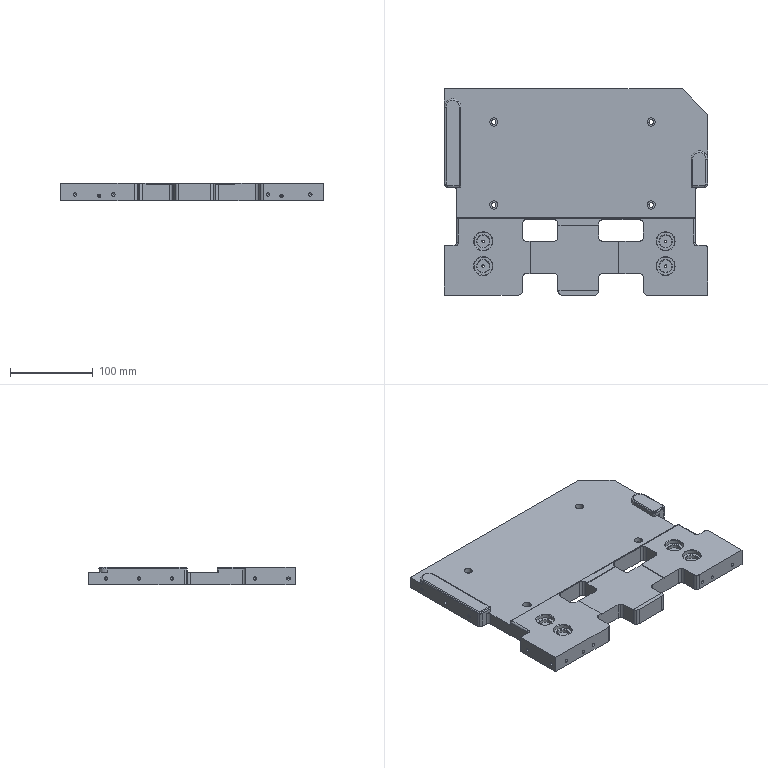Part | STEP file | ASND-0110-TCTF01-35 | 1 solid | 260 faces | box 317.501 x 248.833 x 21 mm | volume 1208594 mm3 | cylinder 150 | plane 55 | cone 42 | torus 9 | sphere 4 | commonest cylinder face diameters 4 x46 10 x40 3 x28 8 x10 5.5 x8 15 x8